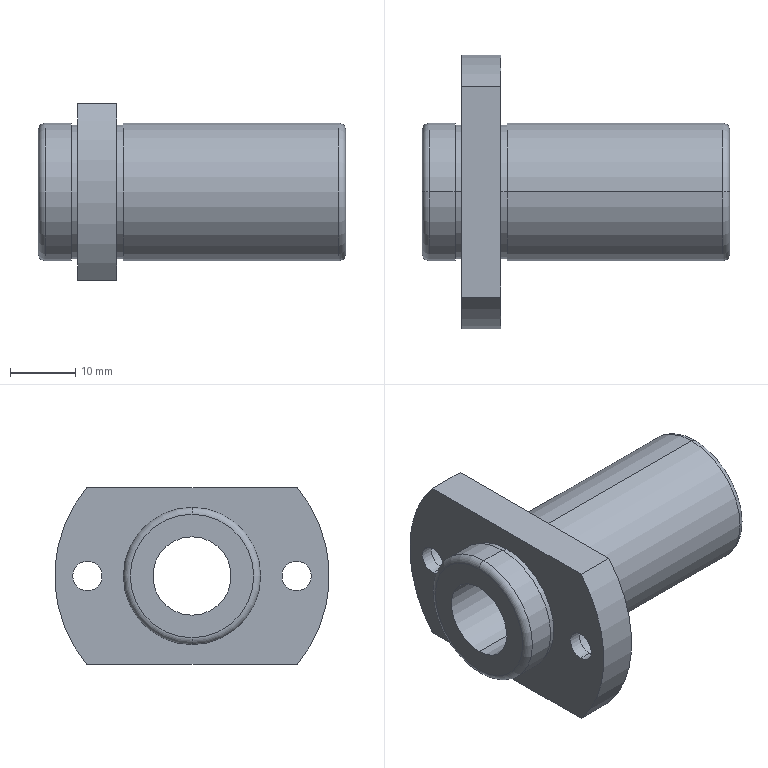Part | STEP file | LHICD12_LHICD12 | 1 solid | 34 faces | box 47 x 42 x 27 mm | volume 14694 mm3 | cylinder 20 | plane 10 | torus 4 | commonest cylinder face diameters 4.5 x4 7.5 x4 20.4 x4 21 x4 12 x2 42 x2